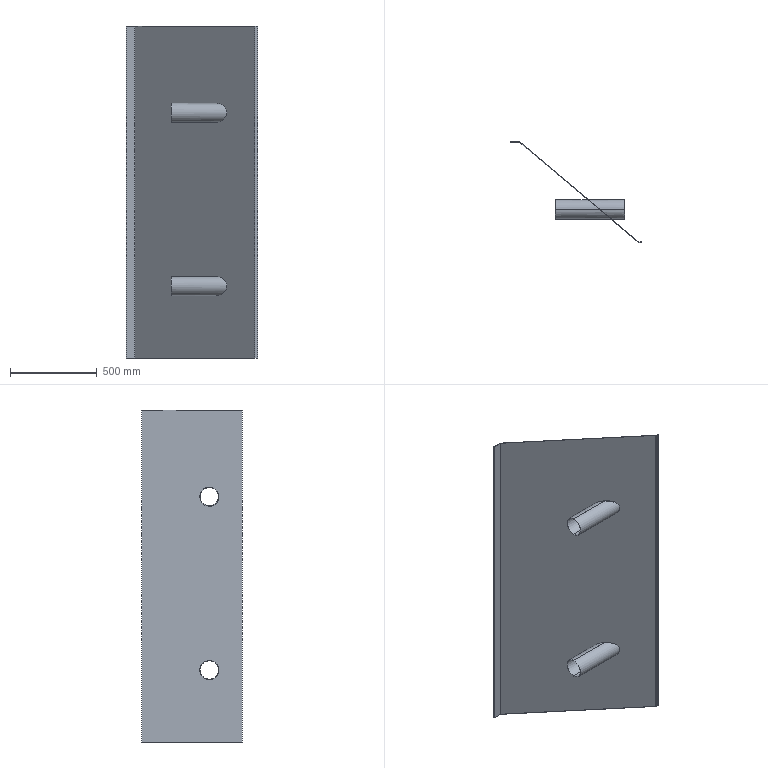Part | SolidWorks | features ICE 2, FlatPattern 1, SMBaseFlange 1, SheetMetal 1 | 1 solid | 38 faces | box 757 x 581.2 x 1915 mm | volume 2731991 mm3 | plane 22 | cylinder 16 | commonest cylinder face diameters 110 x8 106 x4 0.2 x2 2.6 x2
STEP:
#1=CARTESIAN_POINT('',(660.,-390.896,362.));
#2=VERTEX_POINT('',#1);
#3=CARTESIAN_POINT('',(660.,-390.896,468.));
#4=VERTEX_POINT('',#3);
#5=CARTESIAN_POINT('',(660.,-390.896,415.));
#6=DIRECTION('',(-1.,0.,0.));
#7=DIRECTION('',(0.,0.,1.));
#8=AXIS2_PLACEMENT_3D('',#5,#6,#7);
#9=CIRCLE('',#8,53.);
#10=EDGE_CURVE('',#2,#4,#9,.T.);
#11=ORIENTED_EDGE('',*,*,#10,.F.);
#12=CARTESIAN_POINT('',(260.,-390.896,362.));
#13=VERTEX_POINT('',#12);
#14=CARTESIAN_POINT('',(660.,-390.896,362.));
#15=DIRECTION('',(-1.,0.,0.));
#16=VECTOR('',#15,1000.);
#17=LINE('',#14,#16);
#18=EDGE_CURVE('',#2,#13,#17,.T.);
#19=ORIENTED_EDGE('',*,*,#18,.T.);
#20=CARTESIAN_POINT('',(260.,-390.896,468.));
#21=VERTEX_POINT('',#20);
#22=CARTESIAN_POINT('',(260.,-390.896,415.));
#23=DIRECTION('',(-1.,0.,0.));
#24=DIRECTION('',(0.,0.,1.));
#25=AXIS2_PLACEMENT_3D('',#22,#23,#24);
#26=CIRCLE('',#25,53.);
#27=EDGE_CURVE('',#13,#21,#26,.T.);
#28=ORIENTED_EDGE('',*,*,#27,.T.);
#29=CARTESIAN_POINT('',(660.,-390.896,468.));
#30=DIRECTION('',(-1.,0.,0.));
#31=VECTOR('',#30,1000.);
#32=LINE('',#29,#31);
#33=EDGE_CURVE('',#4,#21,#32,.T.);
#34=ORIENTED_EDGE('',*,*,#33,.F.);
#35=EDGE_LOOP('',(#11,#19,#28,#34));
#36=FACE_OUTER_BOUND('',#35,.T.);
#37=CARTESIAN_POINT('',(660.,-390.896,415.));
#38=DIRECTION('',(-1.,0.,0.));
#39=DIRECTION('',(0.,0.,1.));
#40=AXIS2_PLACEMENT_3D('',#37,#38,#39);
#41=CYLINDRICAL_SURFACE('',#40,53.);
#42=ADVANCED_FACE('',(#36),#41,.F.);
#43=CARTESIAN_POINT('',(660.,-390.896,470.));
#44=VERTEX_POINT('',#43);
#45=CARTESIAN_POINT('',(660.,-390.896,360.));
#46=VERTEX_POINT('',#45);
#47=CARTESIAN_POINT('',(660.,-390.896,415.));
#48=DIRECTION('',(-1.,0.,0.));
#49=DIRECTION('',(0.,0.,1.));
#50=AXIS2_PLACEMENT_3D('',#47,#48,#49);
#51=CIRCLE('',#50,55.);
#52=EDGE_CURVE('',#44,#46,#51,.T.);
#53=ORIENTED_EDGE('',*,*,#52,.T.);
#54=CARTESIAN_POINT('',(515.852,-390.896,360.));
#55=VERTEX_POINT('',#54);
#56=CARTESIAN_POINT('',(660.,-390.896,360.));
#57=DIRECTION('',(-1.,0.,0.));
#58=VECTOR('',#57,1000.);
#59=LINE('',#56,#58);
#60=EDGE_CURVE('',#46,#55,#59,.T.);
#61=ORIENTED_EDGE('',*,*,#60,.T.);
#62=CARTESIAN_POINT('',(515.852,-390.896,470.));
#63=VERTEX_POINT('',#62);
#64=CARTESIAN_POINT('',(515.852,-390.896,360.));
#65=CARTESIAN_POINT('',(384.759,-280.896,360.));
#66=CARTESIAN_POINT('',(384.759,-280.896,470.));
#67=CARTESIAN_POINT('',(515.852,-390.896,470.));
#68=(BOUNDED_CURVE()B_SPLINE_CURVE(3,(#64,#65,#66,#67),.UNSPECIFIED.,.F.,.F.)B_SPLINE_CURVE_WITH_KNOTS((4,4),(4.712,7.854),.UNSPECIFIED.)CURVE()GEOMETRIC_REPRESENTATION_ITEM()RATIONAL_B_SPLINE_CURVE((1.,0.3333,0.3333,1.))REPRESENTATION_ITEM(''));
#69=EDGE_CURVE('',#55,#63,#68,.T.);
#70=ORIENTED_EDGE('',*,*,#69,.T.);
#71=CARTESIAN_POINT('',(660.,-390.896,470.));
#72=DIRECTION('',(-1.,0.,0.));
#73=VECTOR('',#72,1000.);
#74=LINE('',#71,#73);
#75=EDGE_CURVE('',#44,#63,#74,.T.);
#76=ORIENTED_EDGE('',*,*,#75,.F.);
#77=EDGE_LOOP('',(#53,#61,#70,#76));
#78=FACE_OUTER_BOUND('',#77,.T.);
#79=CARTESIAN_POINT('',(660.,-390.896,415.));
#80=DIRECTION('',(-1.,0.,0.));
#81=DIRECTION('',(0.,0.,1.));
#82=AXIS2_PLACEMENT_3D('',#79,#80,#81);
#83=CYLINDRICAL_SURFACE('',#82,55.);
#84=ADVANCED_FACE('',(#78),#83,.T.);
#85=CARTESIAN_POINT('',(513.985,-390.896,360.));
#86=VERTEX_POINT('',#85);
#87=CARTESIAN_POINT('',(513.985,-390.896,470.));
#88=VERTEX_POINT('',#87);
#89=CARTESIAN_POINT('',(513.985,-390.896,360.));
#90=CARTESIAN_POINT('',(382.892,-280.896,360.));
#91=CARTESIAN_POINT('',(382.892,-280.896,470.));
#92=CARTESIAN_POINT('',(513.985,-390.896,470.));
#93=(BOUNDED_CURVE()B_SPLINE_CURVE(3,(#89,#90,#91,#92),.UNSPECIFIED.,.F.,.T.)B_SPLINE_CURVE_WITH_KNOTS((4,4),(4.712,7.854),.UNSPECIFIED.)CURVE()GEOMETRIC_REPRESENTATION_ITEM()RATIONAL_B_SPLINE_CURVE((1.,0.3333,0.3333,1.))REPRESENTATION_ITEM(''));
#94=EDGE_CURVE('',#86,#88,#93,.T.);
#95=ORIENTED_EDGE('',*,*,#94,.F.);
#96=CARTESIAN_POINT('',(260.,-390.896,360.));
#97=VERTEX_POINT('',#96);
#98=CARTESIAN_POINT('',(660.,-390.896,360.));
#99=DIRECTION('',(-1.,0.,0.));
#100=VECTOR('',#99,1000.);
#101=LINE('',#98,#100);
#102=EDGE_CURVE('',#86,#97,#101,.T.);
#103=ORIENTED_EDGE('',*,*,#102,.T.);
#104=CARTESIAN_POINT('',(260.,-390.896,470.));
#105=VERTEX_POINT('',#104);
#106=CARTESIAN_POINT('',(260.,-390.896,415.));
#107=DIRECTION('',(-1.,0.,0.));
#108=DIRECTION('',(0.,0.,1.));
#109=AXIS2_PLACEMENT_3D('',#106,#107,#108);
#110=CIRCLE('',#109,55.);
#111=EDGE_CURVE('',#105,#97,#110,.T.);
#112=ORIENTED_EDGE('',*,*,#111,.F.);
#113=CARTESIAN_POINT('',(660.,-390.896,470.));
#114=DIRECTION('',(-1.,0.,0.));
#115=VECTOR('',#114,1000.);
#116=LINE('',#113,#115);
#117=EDGE_CURVE('',#88,#105,#116,.T.);
#118=ORIENTED_EDGE('',*,*,#117,.F.);
#119=EDGE_LOOP('',(#95,#103,#112,#118));
#120=FACE_OUTER_BOUND('',#119,.T.);
#121=CARTESIAN_POINT('',(660.,-390.896,415.));
#122=DIRECTION('',(-1.,0.,0.));
#123=DIRECTION('',(0.,0.,1.));
#124=AXIS2_PLACEMENT_3D('',#121,#122,#123);
#125=CYLINDRICAL_SURFACE('',#124,55.);
#126=ADVANCED_FACE('',(#120),#125,.T.);
#127=CARTESIAN_POINT('',(660.,-390.896,1362.));
#128=VERTEX_POINT('',#127);
#129=CARTESIAN_POINT('',(660.,-390.896,1468.));
#130=VERTEX_POINT('',#129);
#131=CARTESIAN_POINT('',(660.,-390.896,1415.));
#132=DIRECTION('',(-1.,0.,0.));
#133=DIRECTION('',(0.,0.,1.));
#134=AXIS2_PLACEMENT_3D('',#131,#132,#133);
#135=CIRCLE('',#134,53.);
#136=EDGE_CURVE('',#128,#130,#135,.T.);
#137=ORIENTED_EDGE('',*,*,#136,.F.);
#138=CARTESIAN_POINT('',(260.,-390.896,1362.));
#139=VERTEX_POINT('',#138);
#140=CARTESIAN_POINT('',(660.,-390.896,1362.));
#141=DIRECTION('',(-1.,0.,0.));
#142=VECTOR('',#141,1000.);
#143=LINE('',#140,#142);
#144=EDGE_CURVE('',#128,#139,#143,.T.);
#145=ORIENTED_EDGE('',*,*,#144,.T.);
#146=CARTESIAN_POINT('',(260.,-390.896,1468.));
#147=VERTEX_POINT('',#146);
#148=CARTESIAN_POINT('',(260.,-390.896,1415.));
#149=DIRECTION('',(-1.,0.,0.));
#150=DIRECTION('',(0.,0.,1.));
#151=AXIS2_PLACEMENT_3D('',#148,#149,#150);
#152=CIRCLE('',#151,53.);
#153=EDGE_CURVE('',#139,#147,#152,.T.);
#154=ORIENTED_EDGE('',*,*,#153,.T.);
#155=CARTESIAN_POINT('',(660.,-390.896,1468.));
#156=DIRECTION('',(-1.,0.,0.));
#157=VECTOR('',#156,1000.);
#158=LINE('',#155,#157);
#159=EDGE_CURVE('',#130,#147,#158,.T.);
#160=ORIENTED_EDGE('',*,*,#159,.F.);
#161=EDGE_LOOP('',(#137,#145,#154,#160));
#162=FACE_OUTER_BOUND('',#161,.T.);
#163=CARTESIAN_POINT('',(660.,-390.896,1415.));
#164=DIRECTION('',(-1.,0.,0.));
#165=DIRECTION('',(0.,0.,1.));
#166=AXIS2_PLACEMENT_3D('',#163,#164,#165);
#167=CYLINDRICAL_SURFACE('',#166,53.);
#168=ADVANCED_FACE('',(#162),#167,.F.);
#169=CARTESIAN_POINT('',(660.,-390.896,1470.));
#170=VERTEX_POINT('',#169);
#171=CARTESIAN_POINT('',(660.,-390.896,1360.));
#172=VERTEX_POINT('',#171);
#173=CARTESIAN_POINT('',(660.,-390.896,1415.));
#174=DIRECTION('',(-1.,0.,0.));
#175=DIRECTION('',(0.,0.,1.));
#176=AXIS2_PLACEMENT_3D('',#173,#174,#175);
#177=CIRCLE('',#176,55.);
#178=EDGE_CURVE('',#170,#172,#177,.T.);
#179=ORIENTED_EDGE('',*,*,#178,.T.);
#180=CARTESIAN_POINT('',(515.852,-390.896,1360.));
#181=VERTEX_POINT('',#180);
#182=CARTESIAN_POINT('',(660.,-390.896,1360.));
#183=DIRECTION('',(-1.,0.,0.));
#184=VECTOR('',#183,1000.);
#185=LINE('',#182,#184);
#186=EDGE_CURVE('',#172,#181,#185,.T.);
#187=ORIENTED_EDGE('',*,*,#186,.T.);
#188=CARTESIAN_POINT('',(515.852,-390.896,1470.));
#189=VERTEX_POINT('',#188);
#190=CARTESIAN_POINT('',(515.852,-390.896,1360.));
#191=CARTESIAN_POINT('',(384.759,-280.896,1360.));
#192=CARTESIAN_POINT('',(384.759,-280.896,1470.));
#193=CARTESIAN_POINT('',(515.852,-390.896,1470.));
#194=(BOUNDED_CURVE()B_SPLINE_CURVE(3,(#190,#191,#192,#193),.UNSPECIFIED.,.F.,.T.)B_SPLINE_CURVE_WITH_KNOTS((4,4),(4.712,7.854),.UNSPECIFIED.)CURVE()GEOMETRIC_REPRESENTATION_ITEM()RATIONAL_B_SPLINE_CURVE((1.,0.3333,0.3333,1.))REPRESENTATION_ITEM(''));
#195=EDGE_CURVE('',#181,#189,#194,.T.);
#196=ORIENTED_EDGE('',*,*,#195,.T.);
#197=CARTESIAN_POINT('',(660.,-390.896,1470.));
#198=DIRECTION('',(-1.,0.,0.));
#199=VECTOR('',#198,1000.);
#200=LINE('',#197,#199);
#201=EDGE_CURVE('',#170,#189,#200,.T.);
#202=ORIENTED_EDGE('',*,*,#201,.F.);
#203=EDGE_LOOP('',(#179,#187,#196,#202));
#204=FACE_OUTER_BOUND('',#203,.T.);
#205=CARTESIAN_POINT('',(660.,-390.896,1415.));
#206=DIRECTION('',(-1.,0.,0.));
#207=DIRECTION('',(0.,0.,1.));
#208=AXIS2_PLACEMENT_3D('',#205,#206,#207);
#209=CYLINDRICAL_SURFACE('',#208,55.);
#210=ADVANCED_FACE('',(#204),#209,.T.);
#211=CARTESIAN_POINT('',(513.985,-390.896,1360.));
#212=VERTEX_POINT('',#211);
#213=CARTESIAN_POINT('',(513.985,-390.896,1470.));
#214=VERTEX_POINT('',#213);
#215=CARTESIAN_POINT('',(513.985,-390.896,1360.));
#216=CARTESIAN_POINT('',(382.892,-280.896,1360.));
#217=CARTESIAN_POINT('',(382.892,-280.896,1470.));
#218=CARTESIAN_POINT('',(513.985,-390.896,1470.));
#219=(BOUNDED_CURVE()B_SPLINE_CURVE(3,(#215,#216,#217,#218),.UNSPECIFIED.,.F.,.T.)B_SPLINE_CURVE_WITH_KNOTS((4,4),(4.712,7.854),.UNSPECIFIED.)CURVE()GEOMETRIC_REPRESENTATION_ITEM()RATIONAL_B_SPLINE_CURVE((1.,0.3333,0.3333,1.))REPRESENTATION_ITEM(''));
#220=EDGE_CURVE('',#212,#214,#219,.T.);
#221=ORIENTED_EDGE('',*,*,#220,.F.);
#222=CARTESIAN_POINT('',(260.,-390.896,1360.));
#223=VERTEX_POINT('',#222);
#224=CARTESIAN_POINT('',(660.,-390.896,1360.));
#225=DIRECTION('',(-1.,0.,0.));
#226=VECTOR('',#225,1000.);
#227=LINE('',#224,#226);
#228=EDGE_CURVE('',#212,#223,#227,.T.);
#229=ORIENTED_EDGE('',*,*,#228,.T.);
#230=CARTESIAN_POINT('',(260.,-390.896,1470.));
#231=VERTEX_POINT('',#230);
#232=CARTESIAN_POINT('',(260.,-390.896,1415.));
#233=DIRECTION('',(-1.,0.,0.));
#234=DIRECTION('',(0.,0.,1.));
#235=AXIS2_PLACEMENT_3D('',#232,#233,#234);
#236=CIRCLE('',#235,55.);
#237=EDGE_CURVE('',#231,#223,#236,.T.);
#238=ORIENTED_EDGE('',*,*,#237,.F.);
#239=CARTESIAN_POINT('',(660.,-390.896,1470.));
#240=DIRECTION('',(-1.,0.,0.));
#241=VECTOR('',#240,1000.);
#242=LINE('',#239,#241);
#243=EDGE_CURVE('',#214,#231,#242,.T.);
#244=ORIENTED_EDGE('',*,*,#243,.F.);
#245=EDGE_LOOP('',(#221,#229,#238,#244));
#246=FACE_OUTER_BOUND('',#245,.T.);
#247=CARTESIAN_POINT('',(660.,-390.896,1415.));
#248=DIRECTION('',(-1.,0.,0.));
#249=DIRECTION('',(0.,0.,1.));
#250=AXIS2_PLACEMENT_3D('',#247,#248,#249);
#251=CYLINDRICAL_SURFACE('',#250,55.);
#252=ADVANCED_FACE('',(#246),#251,.T.);
#253=CARTESIAN_POINT('',(50.362,-0.3041,1915.));
#254=VERTEX_POINT('',#253);
#255=CARTESIAN_POINT('',(49.591,-1.223,1915.));
#256=VERTEX_POINT('',#255);
#257=CARTESIAN_POINT('',(50.362,-0.3041,1915.));
#258=DIRECTION('',(-0.6428,-0.766,0.));
#259=VECTOR('',#258,1000.);
#260=LINE('',#257,#259);
#261=EDGE_CURVE('',#254,#256,#260,.T.);
#262=ORIENTED_EDGE('',*,*,#261,.F.);
#263=CARTESIAN_POINT('',(49.527,0.,1915.));
#264=VERTEX_POINT('',#263);
#265=CARTESIAN_POINT('',(49.527,-1.3,1915.));
#266=DIRECTION('',(0.,0.,-1.));
#267=DIRECTION('',(1.,0.,0.));
#268=AXIS2_PLACEMENT_3D('',#265,#266,#267);
#269=CIRCLE('',#268,1.3);
#270=EDGE_CURVE('',#264,#254,#269,.T.);
#271=ORIENTED_EDGE('',*,*,#270,.F.);
#272=CARTESIAN_POINT('',(49.527,-1.2,1915.));
#273=VERTEX_POINT('',#272);
#274=CARTESIAN_POINT('',(49.527,-1.2,1915.));
#275=DIRECTION('',(0.,1.,0.));
#276=VECTOR('',#275,1000.);
#277=LINE('',#274,#276);
#278=EDGE_CURVE('',#273,#264,#277,.T.);
#279=ORIENTED_EDGE('',*,*,#278,.F.);
#280=CARTESIAN_POINT('',(49.527,-1.3,1915.));
#281=DIRECTION('',(0.,0.,-1.));
#282=DIRECTION('',(1.,0.,0.));
#283=AXIS2_PLACEMENT_3D('',#280,#281,#282);
#284=CIRCLE('',#283,0.1);
#285=EDGE_CURVE('',#273,#256,#284,.T.);
#286=ORIENTED_EDGE('',*,*,#285,.T.);
#287=EDGE_LOOP('',(#262,#271,#279,#286));
#288=FACE_OUTER_BOUND('',#287,.T.);
#289=CARTESIAN_POINT('',(50.362,-0.3041,1915.));
#290=DIRECTION('',(0.,0.,1.));
#291=DIRECTION('',(1.,0.,0.));
#292=AXIS2_PLACEMENT_3D('',#289,#290,#291);
#293=PLANE('',#292);
#294=ADVANCED_FACE('',(#288),#293,.T.);
#295=CARTESIAN_POINT('',(741.189,-579.977,1915.));
#296=VERTEX_POINT('',#295);
#297=CARTESIAN_POINT('',(50.,0.,1915.));
#298=DIRECTION('',(0.766,-0.6428,0.));
#299=VECTOR('',#298,1000.);
#300=LINE('',#297,#299);
#301=EDGE_CURVE('',#254,#296,#300,.T.);
#302=ORIENTED_EDGE('',*,*,#301,.F.);
#303=ORIENTED_EDGE('',*,*,#261,.T.);
#304=CARTESIAN_POINT('',(740.418,-580.896,1915.));
#305=VERTEX_POINT('',#304);
#306=CARTESIAN_POINT('',(49.229,-0.9193,1915.));
#307=DIRECTION('',(0.766,-0.6428,0.));
#308=VECTOR('',#307,1000.);
#309=LINE('',#306,#308);
#310=EDGE_CURVE('',#256,#305,#309,.T.);
#311=ORIENTED_EDGE('',*,*,#310,.T.);
#312=CARTESIAN_POINT('',(740.418,-580.896,1915.));
#313=DIRECTION('',(0.6428,0.766,0.));
#314=VECTOR('',#313,1000.);
#315=LINE('',#312,#314);
#316=EDGE_CURVE('',#305,#296,#315,.T.);
#317=ORIENTED_EDGE('',*,*,#316,.T.);
#318=EDGE_LOOP('',(#302,#303,#311,#317));
#319=FACE_OUTER_BOUND('',#318,.T.);
#320=CARTESIAN_POINT('',(49.527,-1.2,1915.));
#321=DIRECTION('',(0.,0.,1.));
#322=DIRECTION('',(1.,0.,0.));
#323=AXIS2_PLACEMENT_3D('',#320,#321,#322);
#324=PLANE('',#323);
#325=ADVANCED_FACE('',(#319),#324,.T.);
#326=CARTESIAN_POINT('',(49.527,0.,0.));
#327=VERTEX_POINT('',#326);
#328=CARTESIAN_POINT('',(49.527,-1.2,0.));
#329=VERTEX_POINT('',#328);
#330=CARTESIAN_POINT('',(49.527,0.,0.));
#331=DIRECTION('',(0.,-1.,0.));
#332=VECTOR('',#331,1000.);
#333=LINE('',#330,#332);
#334=EDGE_CURVE('',#327,#329,#333,.T.);
#335=ORIENTED_EDGE('',*,*,#334,.F.);
#336=CARTESIAN_POINT('',(50.362,-0.3041,0.));
#337=VERTEX_POINT('',#336);
#338=CARTESIAN_POINT('',(49.527,-1.3,0.));
#339=DIRECTION('',(0.,0.,-1.));
#340=DIRECTION('',(1.,0.,0.));
#341=AXIS2_PLACEMENT_3D('',#338,#339,#340);
#342=CIRCLE('',#341,1.3);
#343=EDGE_CURVE('',#327,#337,#342,.T.);
#344=ORIENTED_EDGE('',*,*,#343,.T.);
#345=CARTESIAN_POINT('',(49.591,-1.223,0.));
#346=VERTEX_POINT('',#345);
#347=CARTESIAN_POINT('',(49.591,-1.223,0.));
#348=DIRECTION('',(0.6428,0.766,0.));
#349=VECTOR('',#348,1000.);
#350=LINE('',#347,#349);
#351=EDGE_CURVE('',#346,#337,#350,.T.);
#352=ORIENTED_EDGE('',*,*,#351,.F.);
#353=CARTESIAN_POINT('',(49.527,-1.3,0.));
#354=DIRECTION('',(0.,0.,-1.));
#355=DIRECTION('',(1.,0.,0.));
#356=AXIS2_PLACEMENT_3D('',#353,#354,#355);
#357=CIRCLE('',#356,0.1);
#358=EDGE_CURVE('',#329,#346,#357,.T.);
#359=ORIENTED_EDGE('',*,*,#358,.F.);
#360=EDGE_LOOP('',(#335,#344,#352,#359));
#361=FACE_OUTER_BOUND('',#360,.T.);
#362=CARTESIAN_POINT('',(49.527,0.,0.));
#363=DIRECTION('',(0.,0.,-1.));
#364=DIRECTION('',(-1.,0.,0.));
#365=AXIS2_PLACEMENT_3D('',#362,#363,#364);
#366=PLANE('',#365);
#367=ADVANCED_FACE('',(#361),#366,.T.);
#368=CARTESIAN_POINT('',(0.,0.,0.));
#369=VERTEX_POINT('',#368);
#370=CARTESIAN_POINT('',(0.,0.,0.));
#371=DIRECTION('',(1.,0.,0.));
#372=VECTOR('',#371,1000.);
#373=LINE('',#370,#372);
#374=EDGE_CURVE('',#369,#327,#373,.T.);
#375=ORIENTED_EDGE('',*,*,#374,.T.);
#376=ORIENTED_EDGE('',*,*,#334,.T.);
#377=CARTESIAN_POINT('',(0.,-1.2,0.));
#378=VERTEX_POINT('',#377);
#379=CARTESIAN_POINT('',(0.,-1.2,0.));
#380=DIRECTION('',(1.,0.,0.));
#381=VECTOR('',#380,1000.);
#382=LINE('',#379,#381);
#383=EDGE_CURVE('',#378,#329,#382,.T.);
#384=ORIENTED_EDGE('',*,*,#383,.F.);
#385=CARTESIAN_POINT('',(0.,-1.2,0.));
#386=DIRECTION('',(0.,1.,0.));
#387=VECTOR('',#386,1000.);
#388=LINE('',#385,#387);
#389=EDGE_CURVE('',#378,#369,#388,.T.);
#390=ORIENTED_EDGE('',*,*,#389,.T.);
#391=EDGE_LOOP('',(#375,#376,#384,#390));
#392=FACE_OUTER_BOUND('',#391,.T.);
#393=CARTESIAN_POINT('',(49.591,-1.223,0.));
#394=DIRECTION('',(0.,0.,-1.));
#395=DIRECTION('',(-1.,0.,0.));
#396=AXIS2_PLACEMENT_3D('',#393,#394,#395);
#397=PLANE('',#396);
#398=ADVANCED_FACE('',(#392),#397,.T.);
#399=CARTESIAN_POINT('',(741.253,-580.,1915.));
#400=VERTEX_POINT('',#399);
#401=CARTESIAN_POINT('',(741.253,-581.2,1915.));
#402=VERTEX_POINT('',#401);
#403=CARTESIAN_POINT('',(741.253,-580.,1915.));
#404=DIRECTION('',(0.,-1.,0.));
#405=VECTOR('',#404,1000.);
#406=LINE('',#403,#405);
#407=EDGE_CURVE('',#400,#402,#406,.T.);
#408=ORIENTED_EDGE('',*,*,#407,.F.);
#409=CARTESIAN_POINT('',(741.253,-579.9,1915.));
#410=DIRECTION('',(0.,0.,1.));
#411=DIRECTION('',(-1.,0.,0.));
#412=AXIS2_PLACEMENT_3D('',#409,#410,#411);
#413=CIRCLE('',#412,0.1);
#414=EDGE_CURVE('',#296,#400,#413,.T.);
#415=ORIENTED_EDGE('',*,*,#414,.F.);
#416=ORIENTED_EDGE('',*,*,#316,.F.);
#417=CARTESIAN_POINT('',(741.253,-579.9,1915.));
#418=DIRECTION('',(0.,0.,1.));
#419=DIRECTION('',(1.,0.,0.));
#420=AXIS2_PLACEMENT_3D('',#417,#418,#419);
#421=CIRCLE('',#420,1.3);
#422=EDGE_CURVE('',#305,#402,#421,.T.);
#423=ORIENTED_EDGE('',*,*,#422,.T.);
#424=EDGE_LOOP('',(#408,#415,#416,#423));
#425=FACE_OUTER_BOUND('',#424,.T.);
#426=CARTESIAN_POINT('',(741.253,-580.,1915.));
#427=DIRECTION('',(0.,0.,1.));
#428=DIRECTION('',(1.,0.,0.));
#429=AXIS2_PLACEMENT_3D('',#426,#427,#428);
#430=PLANE('',#429);
#431=ADVANCED_FACE('',(#425),#430,.T.);
#432=CARTESIAN_POINT('',(757.,-580.,1915.));
#433=VERTEX_POINT('',#432);
#434=CARTESIAN_POINT('',(741.217,-580.,1915.));
#435=DIRECTION('',(1.,0.,0.));
#436=VECTOR('',#435,1000.);
#437=LINE('',#434,#436);
#438=EDGE_CURVE('',#400,#433,#437,.T.);
#439=ORIENTED_EDGE('',*,*,#438,.F.);
#440=ORIENTED_EDGE('',*,*,#407,.T.);
#441=CARTESIAN_POINT('',(757.,-581.2,1915.));
#442=VERTEX_POINT('',#441);
#443=CARTESIAN_POINT('',(741.217,-581.2,1915.));
#444=DIRECTION('',(1.,0.,0.));
#445=VECTOR('',#444,1000.);
#446=LINE('',#443,#445);
#447=EDGE_CURVE('',#402,#442,#446,.T.);
#448=ORIENTED_EDGE('',*,*,#447,.T.);
#449=CARTESIAN_POINT('',(757.,-580.,1915.));
#450=DIRECTION('',(0.,-1.,0.));
#451=VECTOR('',#450,1000.);
#452=LINE('',#449,#451);
#453=EDGE_CURVE('',#433,#442,#452,.T.);
#454=ORIENTED_EDGE('',*,*,#453,.F.);
#455=EDGE_LOOP('',(#439,#440,#448,#454));
#456=FACE_OUTER_BOUND('',#455,.T.);
#457=CARTESIAN_POINT('',(740.418,-580.896,1915.));
#458=DIRECTION('',(0.,0.,1.));
#459=DIRECTION('',(1.,0.,0.));
#460=AXIS2_PLACEMENT_3D('',#457,#458,#459);
#461=PLANE('',#460);
#462=ADVANCED_FACE('',(#456),#461,.T.);
#463=CARTESIAN_POINT('',(741.189,-579.977,0.));
#464=VERTEX_POINT('',#463);
#465=CARTESIAN_POINT('',(740.418,-580.896,0.));
#466=VERTEX_POINT('',#465);
#467=CARTESIAN_POINT('',(741.189,-579.977,0.));
#468=DIRECTION('',(-0.6428,-0.766,0.));
#469=VECTOR('',#468,1000.);
#470=LINE('',#467,#469);
#471=EDGE_CURVE('',#464,#466,#470,.T.);
#472=ORIENTED_EDGE('',*,*,#471,.F.);
#473=CARTESIAN_POINT('',(741.253,-580.,0.));
#474=VERTEX_POINT('',#473);
#475=CARTESIAN_POINT('',(741.253,-579.9,0.));
#476=DIRECTION('',(0.,0.,1.));
#477=DIRECTION('',(-1.,0.,0.));
#478=AXIS2_PLACEMENT_3D('',#475,#476,#477);
#479=CIRCLE('',#478,0.1);
#480=EDGE_CURVE('',#464,#474,#479,.T.);
#481=ORIENTED_EDGE('',*,*,#480,.T.);
#482=CARTESIAN_POINT('',(741.253,-581.2,0.));
#483=VERTEX_POINT('',#482);
#484=CARTESIAN_POINT('',(741.253,-581.2,0.));
#485=DIRECTION('',(0.,1.,0.));
#486=VECTOR('',#485,1000.);
#487=LINE('',#484,#486);
#488=EDGE_CURVE('',#483,#474,#487,.T.);
#489=ORIENTED_EDGE('',*,*,#488,.F.);
#490=CARTESIAN_POINT('',(741.253,-579.9,0.));
#491=DIRECTION('',(0.,0.,1.));
#492=DIRECTION('',(1.,0.,0.));
#493=AXIS2_PLACEMENT_3D('',#490,#491,#492);
#494=CIRCLE('',#493,1.3);
#495=EDGE_CURVE('',#466,#483,#494,.T.);
#496=ORIENTED_EDGE('',*,*,#495,.F.);
#497=EDGE_LOOP('',(#472,#481,#489,#496));
#498=FACE_OUTER_BOUND('',#497,.T.);
#499=CARTESIAN_POINT('',(741.189,-579.977,0.));
#500=DIRECTION('',(0.,0.,-1.));
#501=DIRECTION('',(-1.,0.,0.));
#502=AXIS2_PLACEMENT_3D('',#499,#500,#501);
#503=PLANE('',#502);
#504=ADVANCED_FACE('',(#498),#503,.T.);
#505=CARTESIAN_POINT('',(50.,0.,0.));
#506=DIRECTION('',(0.766,-0.6428,0.));
#507=VECTOR('',#506,1000.);
#508=LINE('',#505,#507);
#509=EDGE_CURVE('',#337,#464,#508,.T.);
#510=ORIENTED_EDGE('',*,*,#509,.T.);
#511=ORIENTED_EDGE('',*,*,#471,.T.);
#512=CARTESIAN_POINT('',(49.229,-0.9193,0.));
#513=DIRECTION('',(0.766,-0.6428,0.));
#514=VECTOR('',#513,1000.);
#515=LINE('',#512,#514);
#516=EDGE_CURVE('',#346,#466,#515,.T.);
#517=ORIENTED_EDGE('',*,*,#516,.F.);
#518=ORIENTED_EDGE('',*,*,#351,.T.);
#519=EDGE_LOOP('',(#510,#511,#517,#518));
#520=FACE_OUTER_BOUND('',#519,.T.);
#521=CARTESIAN_POINT('',(741.253,-581.2,0.));
#522=DIRECTION('',(0.,0.,-1.));
#523=DIRECTION('',(-1.,0.,0.));
#524=AXIS2_PLACEMENT_3D('',#521,#522,#523);
#525=PLANE('',#524);
#526=ADVANCED_FACE('',(#520),#525,.T.);
#527=CARTESIAN_POINT('',(757.,-581.2,0.));
#528=VERTEX_POINT('',#527);
#529=CARTESIAN_POINT('',(741.217,-581.2,0.));
#530=DIRECTION('',(1.,0.,0.));
#531=VECTOR('',#530,1000.);
#532=LINE('',#529,#531);
#533=EDGE_CURVE('',#483,#528,#532,.T.);
#534=ORIENTED_EDGE('',*,*,#533,.T.);
#535=CARTESIAN_POINT('',(757.,-581.2,1915.));
#536=DIRECTION('',(0.,0.,-1.));
#537=VECTOR('',#536,1000.);
#538=LINE('',#535,#537);
#539=EDGE_CURVE('',#442,#528,#538,.T.);
#540=ORIENTED_EDGE('',*,*,#539,.F.);
#541=ORIENTED_EDGE('',*,*,#447,.F.);
#542=CARTESIAN_POINT('',(741.253,-581.2,1915.));
#543=DIRECTION('',(0.,0.,-1.));
#544=VECTOR('',#543,1000.);
#545=LINE('',#542,#544);
#546=EDGE_CURVE('',#402,#483,#545,.T.);
#547=ORIENTED_EDGE('',*,*,#546,.T.);
#548=EDGE_LOOP('',(#534,#540,#541,#547));
#549=FACE_OUTER_BOUND('',#548,.T.);
#550=CARTESIAN_POINT('',(741.217,-581.2,1915.));
#551=DIRECTION('',(0.,1.,0.));
#552=DIRECTION('',(0.,0.,1.));
#553=AXIS2_PLACEMENT_3D('',#550,#551,#552);
#554=PLANE('',#553);
#555=ADVANCED_FACE('',(#549),#554,.F.);
#556=CARTESIAN_POINT('',(757.,-580.,0.));
#557=VERTEX_POINT('',#556);
#558=CARTESIAN_POINT('',(757.,-580.,0.));
#559=DIRECTION('',(0.,-1.,0.));
#560=VECTOR('',#559,1000.);
#561=LINE('',#558,#560);
#562=EDGE_CURVE('',#557,#528,#561,.T.);
#563=ORIENTED_EDGE('',*,*,#562,.F.);
#564=CARTESIAN_POINT('',(757.,-580.,1915.));
#565=DIRECTION('',(0.,0.,-1.));
#566=VECTOR('',#565,1000.);
#567=LINE('',#564,#566);
#568=EDGE_CURVE('',#433,#557,#567,.T.);
#569=ORIENTED_EDGE('',*,*,#568,.F.);
#570=ORIENTED_EDGE('',*,*,#453,.T.);
#571=ORIENTED_EDGE('',*,*,#539,.T.);
#572=EDGE_LOOP('',(#563,#569,#570,#571));
#573=FACE_OUTER_BOUND('',#572,.T.);
#574=CARTESIAN_POINT('',(757.,-580.,1915.));
#575=DIRECTION('',(1.,0.,0.));
#576=DIRECTION('',(0.,0.,-1.));
#577=AXIS2_PLACEMENT_3D('',#574,#575,#576);
#578=PLANE('',#577);
#579=ADVANCED_FACE('',(#573),#578,.T.);
#580=CARTESIAN_POINT('',(741.217,-580.,0.));
#581=DIRECTION('',(1.,0.,0.));
#582=VECTOR('',#581,1000.);
#583=LINE('',#580,#582);
#584=EDGE_CURVE('',#474,#557,#583,.T.);
#585=ORIENTED_EDGE('',*,*,#584,.F.);
#586=CARTESIAN_POINT('',(741.253,-580.,1915.));
#587=DIRECTION('',(0.,0.,-1.));
#588=VECTOR('',#587,1000.);
#589=LINE('',#586,#588);
#590=EDGE_CURVE('',#400,#474,#589,.T.);
#591=ORIENTED_EDGE('',*,*,#590,.F.);
#592=ORIENTED_EDGE('',*,*,#438,.T.);
#593=ORIENTED_EDGE('',*,*,#568,.T.);
#594=EDGE_LOOP('',(#585,#591,#592,#593));
#595=FACE_OUTER_BOUND('',#594,.T.);
#596=CARTESIAN_POINT('',(741.217,-580.,1915.));
#597=DIRECTION('',(0.,1.,0.));
#598=DIRECTION('',(0.,0.,1.));
#599=AXIS2_PLACEMENT_3D('',#596,#597,#598);
#600=PLANE('',#599);
#601=ADVANCED_FACE('',(#595),#600,.T.);
#602=ORIENTED_EDGE('',*,*,#480,.F.);
#603=CARTESIAN_POINT('',(741.189,-579.977,1915.));
#604=DIRECTION('',(0.,0.,-1.));
#605=VECTOR('',#604,1000.);
#606=LINE('',#603,#605);
#607=EDGE_CURVE('',#296,#464,#606,.T.);
#608=ORIENTED_EDGE('',*,*,#607,.F.);
#609=ORIENTED_EDGE('',*,*,#414,.T.);
#610=ORIENTED_EDGE('',*,*,#590,.T.);
#611=EDGE_LOOP('',(#602,#608,#609,#610));
#612=FACE_OUTER_BOUND('',#611,.T.);
#613=CARTESIAN_POINT('',(741.253,-579.9,1915.));
#614=DIRECTION('',(0.,0.,-1.));
#615=DIRECTION('',(-1.,0.,0.));
#616=AXIS2_PLACEMENT_3D('',#613,#614,#615);
#617=CYLINDRICAL_SURFACE('',#616,0.1);
#618=ADVANCED_FACE('',(#612),#617,.F.);
#619=CARTESIAN_POINT('',(515.852,-390.896,470.));
#620=CARTESIAN_POINT('',(646.944,-500.896,470.));
#621=CARTESIAN_POINT('',(646.944,-500.896,360.));
#622=CARTESIAN_POINT('',(515.852,-390.896,360.));
#623=(BOUNDED_CURVE()B_SPLINE_CURVE(3,(#619,#620,#621,#622),.UNSPECIFIED.,.F.,.T.)B_SPLINE_CURVE_WITH_KNOTS((4,4),(1.571,4.712),.UNSPECIFIED.)CURVE()GEOMETRIC_REPRESENTATION_ITEM()RATIONAL_B_SPLINE_CURVE((1.,0.3333,0.3333,1.))REPRESENTATION_ITEM(''));
#624=EDGE_CURVE('',#63,#55,#623,.T.);
#625=ORIENTED_EDGE('',*,*,#624,.F.);
#626=ORIENTED_EDGE('',*,*,#69,.F.);
#627=EDGE_LOOP('',(#625,#626));
#628=FACE_BOUND('',#627,.T.);
#629=CARTESIAN_POINT('',(515.852,-390.896,1470.));
#630=CARTESIAN_POINT('',(646.944,-500.896,1470.));
#631=CARTESIAN_POINT('',(646.944,-500.896,1360.));
#632=CARTESIAN_POINT('',(515.852,-390.896,1360.));
#633=(BOUNDED_CURVE()B_SPLINE_CURVE(3,(#629,#630,#631,#632),.UNSPECIFIED.,.F.,.F.)B_SPLINE_CURVE_WITH_KNOTS((4,4),(1.571,4.712),.UNSPECIFIED.)CURVE()GEOMETRIC_REPRESENTATION_ITEM()RATIONAL_B_SPLINE_CURVE((1.,0.3333,0.3333,1.))REPRESENTATION_ITEM(''));
#634=EDGE_CURVE('',#189,#181,#633,.T.);
#635=ORIENTED_EDGE('',*,*,#634,.F.);
#636=ORIENTED_EDGE('',*,*,#195,.F.);
#637=EDGE_LOOP('',(#635,#636));
#638=FACE_BOUND('',#637,.T.);
#639=ORIENTED_EDGE('',*,*,#509,.F.);
#640=CARTESIAN_POINT('',(50.362,-0.3041,1915.));
#641=DIRECTION('',(0.,0.,-1.));
#642=VECTOR('',#641,1000.);
#643=LINE('',#640,#642);
#644=EDGE_CURVE('',#254,#337,#643,.T.);
#645=ORIENTED_EDGE('',*,*,#644,.F.);
#646=ORIENTED_EDGE('',*,*,#301,.T.);
#647=ORIENTED_EDGE('',*,*,#607,.T.);
#648=EDGE_LOOP('',(#639,#645,#646,#647));
#649=FACE_OUTER_BOUND('',#648,.T.);
#650=CARTESIAN_POINT('',(50.,0.,1915.));
#651=DIRECTION('',(0.6428,0.766,0.));
#652=DIRECTION('',(-0.766,0.6428,0.));
#653=AXIS2_PLACEMENT_3D('',#650,#651,#652);
#654=PLANE('',#653);
#655=ADVANCED_FACE('',(#628,#638,#649),#654,.T.);
#656=ORIENTED_EDGE('',*,*,#343,.F.);
#657=CARTESIAN_POINT('',(49.527,0.,1915.));
#658=DIRECTION('',(0.,0.,-1.));
#659=VECTOR('',#658,1000.);
#660=LINE('',#657,#659);
#661=EDGE_CURVE('',#264,#327,#660,.T.);
#662=ORIENTED_EDGE('',*,*,#661,.F.);
#663=ORIENTED_EDGE('',*,*,#270,.T.);
#664=ORIENTED_EDGE('',*,*,#644,.T.);
#665=EDGE_LOOP('',(#656,#662,#663,#664));
#666=FACE_OUTER_BOUND('',#665,.T.);
#667=CARTESIAN_POINT('',(49.527,-1.3,1915.));
#668=DIRECTION('',(0.,0.,-1.));
#669=DIRECTION('',(-1.,0.,0.));
#670=AXIS2_PLACEMENT_3D('',#667,#668,#669);
#671=CYLINDRICAL_SURFACE('',#670,1.3);
#672=ADVANCED_FACE('',(#666),#671,.T.);
#673=ORIENTED_EDGE('',*,*,#374,.F.);
#674=CARTESIAN_POINT('',(0.,0.,1915.));
#675=VERTEX_POINT('',#674);
#676=CARTESIAN_POINT('',(0.,0.,1915.));
#677=DIRECTION('',(0.,0.,-1.));
#678=VECTOR('',#677,1000.);
#679=LINE('',#676,#678);
#680=EDGE_CURVE('',#675,#369,#679,.T.);
#681=ORIENTED_EDGE('',*,*,#680,.F.);
#682=CARTESIAN_POINT('',(0.,0.,1915.));
#683=DIRECTION('',(1.,0.,0.));
#684=VECTOR('',#683,1000.);
#685=LINE('',#682,#684);
#686=EDGE_CURVE('',#675,#264,#685,.T.);
#687=ORIENTED_EDGE('',*,*,#686,.T.);
#688=ORIENTED_EDGE('',*,*,#661,.T.);
#689=EDGE_LOOP('',(#673,#681,#687,#688));
#690=FACE_OUTER_BOUND('',#689,.T.);
#691=CARTESIAN_POINT('',(0.,0.,1915.));
#692=DIRECTION('',(0.,1.,0.));
#693=DIRECTION('',(0.,0.,1.));
#694=AXIS2_PLACEMENT_3D('',#691,#692,#693);
#695=PLANE('',#694);
#696=ADVANCED_FACE('',(#690),#695,.T.);
#697=ORIENTED_EDGE('',*,*,#389,.F.);
#698=CARTESIAN_POINT('',(0.,-1.2,1915.));
#699=VERTEX_POINT('',#698);
#700=CARTESIAN_POINT('',(0.,-1.2,1915.));
#701=DIRECTION('',(0.,0.,-1.));
#702=VECTOR('',#701,1000.);
#703=LINE('',#700,#702);
#704=EDGE_CURVE('',#699,#378,#703,.T.);
#705=ORIENTED_EDGE('',*,*,#704,.F.);
#706=CARTESIAN_POINT('',(0.,-1.2,1915.));
#707=DIRECTION('',(0.,1.,0.));
#708=VECTOR('',#707,1000.);
#709=LINE('',#706,#708);
#710=EDGE_CURVE('',#699,#675,#709,.T.);
#711=ORIENTED_EDGE('',*,*,#710,.T.);
#712=ORIENTED_EDGE('',*,*,#680,.T.);
#713=EDGE_LOOP('',(#697,#705,#711,#712));
#714=FACE_OUTER_BOUND('',#713,.T.);
#715=CARTESIAN_POINT('',(0.,-1.2,1915.));
#716=DIRECTION('',(-1.,0.,0.));
#717=DIRECTION('',(0.,0.,1.));
#718=AXIS2_PLACEMENT_3D('',#715,#716,#717);
#719=PLANE('',#718);
#720=ADVANCED_FACE('',(#714),#719,.T.);
#721=ORIENTED_EDGE('',*,*,#383,.T.);
#722=CARTESIAN_POINT('',(49.527,-1.2,1915.));
#723=DIRECTION('',(0.,0.,-1.));
#724=VECTOR('',#723,1000.);
#725=LINE('',#722,#724);
#726=EDGE_CURVE('',#273,#329,#725,.T.);
#727=ORIENTED_EDGE('',*,*,#726,.F.);
#728=CARTESIAN_POINT('',(0.,-1.2,1915.));
#729=DIRECTION('',(1.,0.,0.));
#730=VECTOR('',#729,1000.);
#731=LINE('',#728,#730);
#732=EDGE_CURVE('',#699,#273,#731,.T.);
#733=ORIENTED_EDGE('',*,*,#732,.F.);
#734=ORIENTED_EDGE('',*,*,#704,.T.);
#735=EDGE_LOOP('',(#721,#727,#733,#734));
#736=FACE_OUTER_BOUND('',#735,.T.);
#737=CARTESIAN_POINT('',(0.,-1.2,1915.));
#738=DIRECTION('',(0.,1.,0.));
#739=DIRECTION('',(0.,0.,1.));
#740=AXIS2_PLACEMENT_3D('',#737,#738,#739);
#741=PLANE('',#740);
#742=ADVANCED_FACE('',(#736),#741,.F.);
#743=ORIENTED_EDGE('',*,*,#358,.T.);
#744=CARTESIAN_POINT('',(49.591,-1.223,1915.));
#745=DIRECTION('',(0.,0.,-1.));
#746=VECTOR('',#745,1000.);
#747=LINE('',#744,#746);
#748=EDGE_CURVE('',#256,#346,#747,.T.);
#749=ORIENTED_EDGE('',*,*,#748,.F.);
#750=ORIENTED_EDGE('',*,*,#285,.F.);
#751=ORIENTED_EDGE('',*,*,#726,.T.);
#752=EDGE_LOOP('',(#743,#749,#750,#751));
#753=FACE_OUTER_BOUND('',#752,.T.);
#754=CARTESIAN_POINT('',(49.527,-1.3,1915.));
#755=DIRECTION('',(0.,0.,-1.));
#756=DIRECTION('',(-1.,0.,0.));
#757=AXIS2_PLACEMENT_3D('',#754,#755,#756);
#758=CYLINDRICAL_SURFACE('',#757,0.1);
#759=ADVANCED_FACE('',(#753),#758,.F.);
#760=CARTESIAN_POINT('',(513.985,-390.896,470.));
#761=CARTESIAN_POINT('',(645.078,-500.896,470.));
#762=CARTESIAN_POINT('',(645.078,-500.896,360.));
#763=CARTESIAN_POINT('',(513.985,-390.896,360.));
#764=(BOUNDED_CURVE()B_SPLINE_CURVE(3,(#760,#761,#762,#763),.UNSPECIFIED.,.F.,.F.)B_SPLINE_CURVE_WITH_KNOTS((4,4),(1.571,4.712),.UNSPECIFIED.)CURVE()GEOMETRIC_REPRESENTATION_ITEM()RATIONAL_B_SPLINE_CURVE((1.,0.3333,0.3333,1.))REPRESENTATION_ITEM(''));
#765=EDGE_CURVE('',#88,#86,#764,.T.);
#766=ORIENTED_EDGE('',*,*,#765,.T.);
#767=ORIENTED_EDGE('',*,*,#94,.T.);
#768=EDGE_LOOP('',(#766,#767));
#769=FACE_BOUND('',#768,.T.);
#770=CARTESIAN_POINT('',(513.985,-390.896,1470.));
#771=CARTESIAN_POINT('',(645.078,-500.896,1470.));
#772=CARTESIAN_POINT('',(645.078,-500.896,1360.));
#773=CARTESIAN_POINT('',(513.985,-390.896,1360.));
#774=(BOUNDED_CURVE()B_SPLINE_CURVE(3,(#770,#771,#772,#773),.UNSPECIFIED.,.F.,.T.)B_SPLINE_CURVE_WITH_KNOTS((4,4),(1.571,4.712),.UNSPECIFIED.)CURVE()GEOMETRIC_REPRESENTATION_ITEM()RATIONAL_B_SPLINE_CURVE((1.,0.3333,0.3333,1.))REPRESENTATION_ITEM(''));
#775=EDGE_CURVE('',#214,#212,#774,.T.);
#776=ORIENTED_EDGE('',*,*,#775,.T.);
#777=ORIENTED_EDGE('',*,*,#220,.T.);
#778=EDGE_LOOP('',(#776,#777));
#779=FACE_BOUND('',#778,.T.);
#780=ORIENTED_EDGE('',*,*,#516,.T.);
#781=CARTESIAN_POINT('',(740.418,-580.896,1915.));
#782=DIRECTION('',(0.,0.,-1.));
#783=VECTOR('',#782,1000.);
#784=LINE('',#781,#783);
#785=EDGE_CURVE('',#305,#466,#784,.T.);
#786=ORIENTED_EDGE('',*,*,#785,.F.);
#787=ORIENTED_EDGE('',*,*,#310,.F.);
#788=ORIENTED_EDGE('',*,*,#748,.T.);
#789=EDGE_LOOP('',(#780,#786,#787,#788));
#790=FACE_OUTER_BOUND('',#789,.T.);
#791=CARTESIAN_POINT('',(49.229,-0.9193,1915.));
#792=DIRECTION('',(0.6428,0.766,0.));
#793=DIRECTION('',(-0.766,0.6428,0.));
#794=AXIS2_PLACEMENT_3D('',#791,#792,#793);
#795=PLANE('',#794);
#796=ADVANCED_FACE('',(#769,#779,#790),#795,.F.);
#797=ORIENTED_EDGE('',*,*,#495,.T.);
#798=ORIENTED_EDGE('',*,*,#546,.F.);
#799=ORIENTED_EDGE('',*,*,#422,.F.);
#800=ORIENTED_EDGE('',*,*,#785,.T.);
#801=EDGE_LOOP('',(#797,#798,#799,#800));
#802=FACE_OUTER_BOUND('',#801,.T.);
#803=CARTESIAN_POINT('',(741.253,-579.9,1915.));
#804=DIRECTION('',(0.,0.,-1.));
#805=DIRECTION('',(-1.,0.,0.));
#806=AXIS2_PLACEMENT_3D('',#803,#804,#805);
#807=CYLINDRICAL_SURFACE('',#806,1.3);
#808=ADVANCED_FACE('',(#802),#807,.T.);
#809=ORIENTED_EDGE('',*,*,#732,.T.);
#810=ORIENTED_EDGE('',*,*,#278,.T.);
#811=ORIENTED_EDGE('',*,*,#686,.F.);
#812=ORIENTED_EDGE('',*,*,#710,.F.);
#813=EDGE_LOOP('',(#809,#810,#811,#812));
#814=FACE_OUTER_BOUND('',#813,.T.);
#815=CARTESIAN_POINT('',(741.253,-579.9,1915.));
#816=DIRECTION('',(0.,0.,-1.));
#817=DIRECTION('',(-1.,0.,0.));
#818=AXIS2_PLACEMENT_3D('',#815,#816,#817);
#819=PLANE('',#818);
#820=ADVANCED_FACE('',(#814),#819,.F.);
#821=ORIENTED_EDGE('',*,*,#533,.F.);
#822=ORIENTED_EDGE('',*,*,#488,.T.);
#823=ORIENTED_EDGE('',*,*,#584,.T.);
#824=ORIENTED_EDGE('',*,*,#562,.T.);
#825=EDGE_LOOP('',(#821,#822,#823,#824));
#826=FACE_OUTER_BOUND('',#825,.T.);
#827=CARTESIAN_POINT('',(741.253,-579.9,0.));
#828=DIRECTION('',(0.,0.,-1.));
#829=DIRECTION('',(-1.,0.,0.));
#830=AXIS2_PLACEMENT_3D('',#827,#828,#829);
#831=PLANE('',#830);
#832=ADVANCED_FACE('',(#826),#831,.T.);
#833=ORIENTED_EDGE('',*,*,#228,.F.);
#834=ORIENTED_EDGE('',*,*,#775,.F.);
#835=ORIENTED_EDGE('',*,*,#243,.T.);
#836=CARTESIAN_POINT('',(260.,-390.896,1415.));
#837=DIRECTION('',(-1.,0.,0.));
#838=DIRECTION('',(0.,0.,1.));
#839=AXIS2_PLACEMENT_3D('',#836,#837,#838);
#840=CIRCLE('',#839,55.);
#841=EDGE_CURVE('',#223,#231,#840,.T.);
#842=ORIENTED_EDGE('',*,*,#841,.F.);
#843=EDGE_LOOP('',(#833,#834,#835,#842));
#844=FACE_OUTER_BOUND('',#843,.T.);
#845=CARTESIAN_POINT('',(660.,-390.896,1415.));
#846=DIRECTION('',(-1.,0.,0.));
#847=DIRECTION('',(0.,0.,1.));
#848=AXIS2_PLACEMENT_3D('',#845,#846,#847);
#849=CYLINDRICAL_SURFACE('',#848,55.);
#850=ADVANCED_FACE('',(#844),#849,.T.);
#851=ORIENTED_EDGE('',*,*,#186,.F.);
#852=CARTESIAN_POINT('',(660.,-390.896,1415.));
#853=DIRECTION('',(-1.,0.,0.));
#854=DIRECTION('',(0.,0.,1.));
#855=AXIS2_PLACEMENT_3D('',#852,#853,#854);
#856=CIRCLE('',#855,55.);
#857=EDGE_CURVE('',#172,#170,#856,.T.);
#858=ORIENTED_EDGE('',*,*,#857,.T.);
#859=ORIENTED_EDGE('',*,*,#201,.T.);
#860=ORIENTED_EDGE('',*,*,#634,.T.);
#861=EDGE_LOOP('',(#851,#858,#859,#860));
#862=FACE_OUTER_BOUND('',#861,.T.);
#863=CARTESIAN_POINT('',(660.,-390.896,1415.));
#864=DIRECTION('',(-1.,0.,0.));
#865=DIRECTION('',(0.,0.,1.));
#866=AXIS2_PLACEMENT_3D('',#863,#864,#865);
#867=CYLINDRICAL_SURFACE('',#866,55.);
#868=ADVANCED_FACE('',(#862),#867,.T.);
#869=CARTESIAN_POINT('',(660.,-390.896,1415.));
#870=DIRECTION('',(-1.,0.,0.));
#871=DIRECTION('',(0.,0.,1.));
#872=AXIS2_PLACEMENT_3D('',#869,#870,#871);
#873=CIRCLE('',#872,53.);
#874=EDGE_CURVE('',#130,#128,#873,.T.);
#875=ORIENTED_EDGE('',*,*,#874,.T.);
#876=ORIENTED_EDGE('',*,*,#136,.T.);
#877=EDGE_LOOP('',(#875,#876));
#878=FACE_BOUND('',#877,.T.);
#879=ORIENTED_EDGE('',*,*,#178,.F.);
#880=ORIENTED_EDGE('',*,*,#857,.F.);
#881=EDGE_LOOP('',(#879,#880));
#882=FACE_OUTER_BOUND('',#881,.T.);
#883=CARTESIAN_POINT('',(660.,-390.896,1415.));
#884=DIRECTION('',(-1.,0.,0.));
#885=DIRECTION('',(0.,0.,1.));
#886=AXIS2_PLACEMENT_3D('',#883,#884,#885);
#887=PLANE('',#886);
#888=ADVANCED_FACE('',(#878,#882),#887,.F.);
#889=CARTESIAN_POINT('',(260.,-390.896,1415.));
#890=DIRECTION('',(-1.,0.,0.));
#891=DIRECTION('',(0.,0.,1.));
#892=AXIS2_PLACEMENT_3D('',#889,#890,#891);
#893=CIRCLE('',#892,53.);
#894=EDGE_CURVE('',#147,#139,#893,.T.);
#895=ORIENTED_EDGE('',*,*,#894,.F.);
#896=ORIENTED_EDGE('',*,*,#153,.F.);
#897=EDGE_LOOP('',(#895,#896));
#898=FACE_BOUND('',#897,.T.);
#899=ORIENTED_EDGE('',*,*,#237,.T.);
#900=ORIENTED_EDGE('',*,*,#841,.T.);
#901=EDGE_LOOP('',(#899,#900));
#902=FACE_OUTER_BOUND('',#901,.T.);
#903=CARTESIAN_POINT('',(260.,-390.896,1415.));
#904=DIRECTION('',(-1.,0.,0.));
#905=DIRECTION('',(0.,0.,1.));
#906=AXIS2_PLACEMENT_3D('',#903,#904,#905);
#907=PLANE('',#906);
#908=ADVANCED_FACE('',(#898,#902),#907,.T.);
#909=ORIENTED_EDGE('',*,*,#144,.F.);
#910=ORIENTED_EDGE('',*,*,#874,.F.);
#911=ORIENTED_EDGE('',*,*,#159,.T.);
#912=ORIENTED_EDGE('',*,*,#894,.T.);
#913=EDGE_LOOP('',(#909,#910,#911,#912));
#914=FACE_OUTER_BOUND('',#913,.T.);
#915=CARTESIAN_POINT('',(660.,-390.896,1415.));
#916=DIRECTION('',(-1.,0.,0.));
#917=DIRECTION('',(0.,0.,1.));
#918=AXIS2_PLACEMENT_3D('',#915,#916,#917);
#919=CYLINDRICAL_SURFACE('',#918,53.);
#920=ADVANCED_FACE('',(#914),#919,.F.);
#921=ORIENTED_EDGE('',*,*,#102,.F.);
#922=ORIENTED_EDGE('',*,*,#765,.F.);
#923=ORIENTED_EDGE('',*,*,#117,.T.);
#924=CARTESIAN_POINT('',(260.,-390.896,415.));
#925=DIRECTION('',(-1.,0.,0.));
#926=DIRECTION('',(0.,0.,1.));
#927=AXIS2_PLACEMENT_3D('',#924,#925,#926);
#928=CIRCLE('',#927,55.);
#929=EDGE_CURVE('',#97,#105,#928,.T.);
#930=ORIENTED_EDGE('',*,*,#929,.F.);
#931=EDGE_LOOP('',(#921,#922,#923,#930));
#932=FACE_OUTER_BOUND('',#931,.T.);
#933=CARTESIAN_POINT('',(660.,-390.896,415.));
#934=DIRECTION('',(-1.,0.,0.));
#935=DIRECTION('',(0.,0.,1.));
#936=AXIS2_PLACEMENT_3D('',#933,#934,#935);
#937=CYLINDRICAL_SURFACE('',#936,55.);
#938=ADVANCED_FACE('',(#932),#937,.T.);
#939=ORIENTED_EDGE('',*,*,#60,.F.);
#940=CARTESIAN_POINT('',(660.,-390.896,415.));
#941=DIRECTION('',(-1.,0.,0.));
#942=DIRECTION('',(0.,0.,1.));
#943=AXIS2_PLACEMENT_3D('',#940,#941,#942);
#944=CIRCLE('',#943,55.);
#945=EDGE_CURVE('',#46,#44,#944,.T.);
#946=ORIENTED_EDGE('',*,*,#945,.T.);
#947=ORIENTED_EDGE('',*,*,#75,.T.);
#948=ORIENTED_EDGE('',*,*,#624,.T.);
#949=EDGE_LOOP('',(#939,#946,#947,#948));
#950=FACE_OUTER_BOUND('',#949,.T.);
#951=CARTESIAN_POINT('',(660.,-390.896,415.));
#952=DIRECTION('',(-1.,0.,0.));
#953=DIRECTION('',(0.,0.,1.));
#954=AXIS2_PLACEMENT_3D('',#951,#952,#953);
#955=CYLINDRICAL_SURFACE('',#954,55.);
#956=ADVANCED_FACE('',(#950),#955,.T.);
#957=CARTESIAN_POINT('',(660.,-390.896,415.));
#958=DIRECTION('',(-1.,0.,0.));
#959=DIRECTION('',(0.,0.,1.));
#960=AXIS2_PLACEMENT_3D('',#957,#958,#959);
#961=CIRCLE('',#960,53.);
#962=EDGE_CURVE('',#4,#2,#961,.T.);
#963=ORIENTED_EDGE('',*,*,#962,.T.);
#964=ORIENTED_EDGE('',*,*,#10,.T.);
#965=EDGE_LOOP('',(#963,#964));
#966=FACE_BOUND('',#965,.T.);
#967=ORIENTED_EDGE('',*,*,#52,.F.);
#968=ORIENTED_EDGE('',*,*,#945,.F.);
#969=EDGE_LOOP('',(#967,#968));
#970=FACE_OUTER_BOUND('',#969,.T.);
#971=CARTESIAN_POINT('',(660.,-390.896,415.));
#972=DIRECTION('',(-1.,0.,0.));
#973=DIRECTION('',(0.,0.,1.));
#974=AXIS2_PLACEMENT_3D('',#971,#972,#973);
#975=PLANE('',#974);
#976=ADVANCED_FACE('',(#966,#970),#975,.F.);
#977=CARTESIAN_POINT('',(260.,-390.896,415.));
#978=DIRECTION('',(-1.,0.,0.));
#979=DIRECTION('',(0.,0.,1.));
#980=AXIS2_PLACEMENT_3D('',#977,#978,#979);
#981=CIRCLE('',#980,53.);
#982=EDGE_CURVE('',#21,#13,#981,.T.);
#983=ORIENTED_EDGE('',*,*,#982,.F.);
#984=ORIENTED_EDGE('',*,*,#27,.F.);
#985=EDGE_LOOP('',(#983,#984));
#986=FACE_BOUND('',#985,.T.);
#987=ORIENTED_EDGE('',*,*,#111,.T.);
#988=ORIENTED_EDGE('',*,*,#929,.T.);
#989=EDGE_LOOP('',(#987,#988));
#990=FACE_OUTER_BOUND('',#989,.T.);
#991=CARTESIAN_POINT('',(260.,-390.896,415.));
#992=DIRECTION('',(-1.,0.,0.));
#993=DIRECTION('',(0.,0.,1.));
#994=AXIS2_PLACEMENT_3D('',#991,#992,#993);
#995=PLANE('',#994);
#996=ADVANCED_FACE('',(#986,#990),#995,.T.);
#997=ORIENTED_EDGE('',*,*,#18,.F.);
#998=ORIENTED_EDGE('',*,*,#962,.F.);
#999=ORIENTED_EDGE('',*,*,#33,.T.);
#1000=ORIENTED_EDGE('',*,*,#982,.T.);
#1001=EDGE_LOOP('',(#997,#998,#999,#1000));
#1002=FACE_OUTER_BOUND('',#1001,.T.);
#1003=CARTESIAN_POINT('',(660.,-390.896,415.));
#1004=DIRECTION('',(-1.,0.,0.));
#1005=DIRECTION('',(0.,0.,1.));
#1006=AXIS2_PLACEMENT_3D('',#1003,#1004,#1005);
#1007=CYLINDRICAL_SURFACE('',#1006,53.);
#1008=ADVANCED_FACE('',(#1002),#1007,.F.);
#1009=CLOSED_SHELL('',(#42,#84,#126,#168,#210,#252,#294,#325,#367,#398,#431,#462,#504,#526,#555,#579,#601,#618,#655,#672,#696,#720,#742,#759,#796,#808,#820,#832,#850,#868,#888,#908,#920,#938,#956,#976,#996,#1008));
#1010=MANIFOLD_SOLID_BREP('',#1009);
#1011=CARTESIAN_POINT('',(0.,0.,0.));
#1012=DIRECTION('',(0.,0.,1.));
#1013=DIRECTION('',(1.,0.,0.));
#1014=AXIS2_PLACEMENT_3D('',#1011,#1012,#1013);
#1015=(LENGTH_UNIT()NAMED_UNIT(*)SI_UNIT(.MILLI.,.METRE.));
#1016=UNCERTAINTY_MEASURE_WITH_UNIT(LENGTH_MEASURE(0.00001),#1015,'','');
#1017=(NAMED_UNIT(*)PLANE_ANGLE_UNIT()SI_UNIT($,.RADIAN.));
#1018=(NAMED_UNIT(*)SI_UNIT($,.STERADIAN.)SOLID_ANGLE_UNIT());
#1019=(GEOMETRIC_REPRESENTATION_CONTEXT(3)GLOBAL_UNCERTAINTY_ASSIGNED_CONTEXT((#1016))GLOBAL_UNIT_ASSIGNED_CONTEXT((#1015,#1017,#1018))REPRESENTATION_CONTEXT('',''));
#1020=ADVANCED_BREP_SHAPE_REPRESENTATION('',(#1010,#1014),#1019);